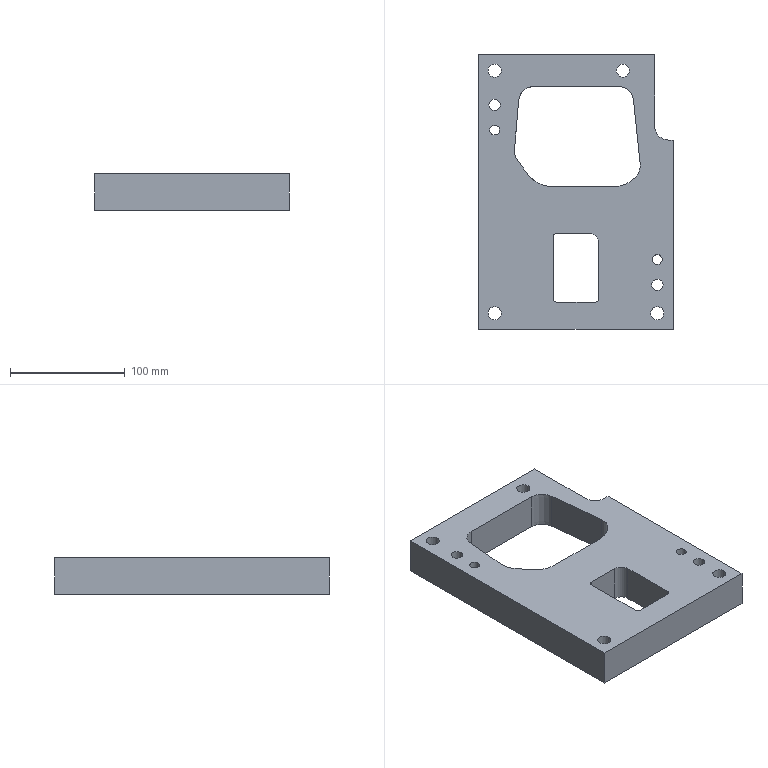Part | STEP file | lll_id3682_x_t | 1 solid | 45 faces | box 170 x 240 x 32 mm | volume 880662 mm3 | plane 22 | cylinder 19 | other 4 | commonest cylinder face diameters 11.509 x4 18.008 x4 6 x3 8.506 x2 10 x2 16 x1
STEP:
#1=CARTESIAN_POINT('',(3672.243,-109.5,60.5));
#2=VERTEX_POINT('',#1);
#3=CARTESIAN_POINT('',(3668.,-109.5,60.5));
#4=VERTEX_POINT('',#3);
#5=CARTESIAN_POINT('',(3587.243,-109.5,60.5));
#6=DIRECTION('',(-1.,0.,0.));
#7=VECTOR('',#6,1.);
#8=LINE('',#5,#7);
#9=EDGE_CURVE('',#2,#4,#8,.T.);
#10=ORIENTED_EDGE('',*,*,#9,.F.);
#11=CARTESIAN_POINT('',(3672.243,-274.803,60.5));
#12=VERTEX_POINT('',#11);
#13=CARTESIAN_POINT('',(3672.243,-156.803,60.5));
#14=DIRECTION('',(0.,-1.,0.));
#15=VECTOR('',#14,1.);
#16=LINE('',#13,#15);
#17=EDGE_CURVE('',#2,#12,#16,.T.);
#18=ORIENTED_EDGE('',*,*,#17,.T.);
#19=CARTESIAN_POINT('',(3502.243,-274.803,60.5));
#20=VERTEX_POINT('',#19);
#21=CARTESIAN_POINT('',(3587.243,-274.803,60.5));
#22=DIRECTION('',(-1.,0.,0.));
#23=VECTOR('',#22,1.);
#24=LINE('',#21,#23);
#25=EDGE_CURVE('',#12,#20,#24,.T.);
#26=ORIENTED_EDGE('',*,*,#25,.T.);
#27=CARTESIAN_POINT('',(3502.243,-34.803,60.5));
#28=VERTEX_POINT('',#27);
#29=CARTESIAN_POINT('',(3502.243,-156.803,60.5));
#30=DIRECTION('',(0.,1.,0.));
#31=VECTOR('',#30,1.);
#32=LINE('',#29,#31);
#33=EDGE_CURVE('',#20,#28,#32,.T.);
#34=ORIENTED_EDGE('',*,*,#33,.T.);
#35=CARTESIAN_POINT('',(3656.,-34.803,60.5));
#36=VERTEX_POINT('',#35);
#37=CARTESIAN_POINT('',(3587.243,-34.803,60.5));
#38=DIRECTION('',(1.,0.,0.));
#39=VECTOR('',#38,1.);
#40=LINE('',#37,#39);
#41=EDGE_CURVE('',#28,#36,#40,.T.);
#42=ORIENTED_EDGE('',*,*,#41,.T.);
#43=CARTESIAN_POINT('',(3656.,-97.5,60.5));
#44=VERTEX_POINT('',#43);
#45=CARTESIAN_POINT('',(3656.,-156.803,60.5));
#46=DIRECTION('',(0.,1.,0.));
#47=VECTOR('',#46,1.);
#48=LINE('',#45,#47);
#49=EDGE_CURVE('',#44,#36,#48,.T.);
#50=ORIENTED_EDGE('',*,*,#49,.F.);
#51=CARTESIAN_POINT('',(3668.,-97.5,60.5));
#52=DIRECTION('',(0.,0.,1.));
#53=DIRECTION('',(-1.,0.,0.));
#54=AXIS2_PLACEMENT_3D('',#51,#52,#53);
#55=CIRCLE('',#54,12.);
#56=EDGE_CURVE('',#44,#4,#55,.T.);
#57=ORIENTED_EDGE('',*,*,#56,.T.);
#58=EDGE_LOOP('',(#10,#18,#26,#34,#42,#50,#57));
#59=FACE_BOUND('',#58,.T.);
#60=CARTESIAN_POINT('',(3511.99,-100.803,60.5));
#61=VERTEX_POINT('',#60);
#62=CARTESIAN_POINT('',(3516.243,-100.803,60.5));
#63=DIRECTION('',(0.,0.,-1.));
#64=DIRECTION('',(-1.,0.,0.));
#65=AXIS2_PLACEMENT_3D('',#62,#63,#64);
#66=CIRCLE('',#65,4.253);
#67=EDGE_CURVE('',#61,#61,#66,.T.);
#68=ORIENTED_EDGE('',*,*,#67,.F.);
#69=EDGE_LOOP('',(#68));
#70=FACE_BOUND('',#69,.T.);
#71=CARTESIAN_POINT('',(3521.244,-78.803,60.5));
#72=VERTEX_POINT('',#71);
#73=CARTESIAN_POINT('',(3516.243,-78.803,60.5));
#74=DIRECTION('',(0.,0.,1.));
#75=DIRECTION('',(1.,0.,0.));
#76=AXIS2_PLACEMENT_3D('',#73,#74,#75);
#77=CIRCLE('',#76,5.);
#78=EDGE_CURVE('',#72,#72,#77,.T.);
#79=ORIENTED_EDGE('',*,*,#78,.T.);
#80=EDGE_LOOP('',(#79));
#81=FACE_BOUND('',#80,.T.);
#82=CARTESIAN_POINT('',(3663.244,-235.803,60.5));
#83=VERTEX_POINT('',#82);
#84=CARTESIAN_POINT('',(3658.243,-235.803,60.5));
#85=DIRECTION('',(0.,0.,1.));
#86=DIRECTION('',(1.,0.,0.));
#87=AXIS2_PLACEMENT_3D('',#84,#85,#86);
#88=CIRCLE('',#87,5.);
#89=EDGE_CURVE('',#83,#83,#88,.T.);
#90=ORIENTED_EDGE('',*,*,#89,.T.);
#91=EDGE_LOOP('',(#90));
#92=FACE_BOUND('',#91,.T.);
#93=CARTESIAN_POINT('',(3507.239,-260.803,60.5));
#94=VERTEX_POINT('',#93);
#95=CARTESIAN_POINT('',(3516.243,-260.803,60.5));
#96=DIRECTION('',(0.,0.,-1.));
#97=DIRECTION('',(-1.,0.,0.));
#98=AXIS2_PLACEMENT_3D('',#95,#96,#97);
#99=CIRCLE('',#98,9.004);
#100=EDGE_CURVE('',#94,#94,#99,.T.);
#101=ORIENTED_EDGE('',*,*,#100,.F.);
#102=EDGE_LOOP('',(#101));
#103=FACE_BOUND('',#102,.T.);
#104=CARTESIAN_POINT('',(3649.239,-260.803,60.5));
#105=VERTEX_POINT('',#104);
#106=CARTESIAN_POINT('',(3658.243,-260.803,60.5));
#107=DIRECTION('',(0.,0.,-1.));
#108=DIRECTION('',(-1.,0.,0.));
#109=AXIS2_PLACEMENT_3D('',#106,#107,#108);
#110=CIRCLE('',#109,9.004);
#111=EDGE_CURVE('',#105,#105,#110,.T.);
#112=ORIENTED_EDGE('',*,*,#111,.F.);
#113=EDGE_LOOP('',(#112));
#114=FACE_BOUND('',#113,.T.);
#115=CARTESIAN_POINT('',(3507.239,-48.803,60.5));
#116=VERTEX_POINT('',#115);
#117=CARTESIAN_POINT('',(3516.243,-48.803,60.5));
#118=DIRECTION('',(0.,0.,-1.));
#119=DIRECTION('',(-1.,0.,0.));
#120=AXIS2_PLACEMENT_3D('',#117,#118,#119);
#121=CIRCLE('',#120,9.004);
#122=EDGE_CURVE('',#116,#116,#121,.T.);
#123=ORIENTED_EDGE('',*,*,#122,.F.);
#124=EDGE_LOOP('',(#123));
#125=FACE_BOUND('',#124,.T.);
#126=CARTESIAN_POINT('',(3619.239,-48.803,60.5));
#127=VERTEX_POINT('',#126);
#128=CARTESIAN_POINT('',(3628.243,-48.803,60.5));
#129=DIRECTION('',(0.,0.,-1.));
#130=DIRECTION('',(-1.,0.,0.));
#131=AXIS2_PLACEMENT_3D('',#128,#129,#130);
#132=CIRCLE('',#131,9.004);
#133=EDGE_CURVE('',#127,#127,#132,.T.);
#134=ORIENTED_EDGE('',*,*,#133,.F.);
#135=EDGE_LOOP('',(#134));
#136=FACE_BOUND('',#135,.T.);
#137=CARTESIAN_POINT('',(3653.99,-213.803,60.5));
#138=VERTEX_POINT('',#137);
#139=CARTESIAN_POINT('',(3658.243,-213.803,60.5));
#140=DIRECTION('',(0.,0.,-1.));
#141=DIRECTION('',(-1.,0.,0.));
#142=AXIS2_PLACEMENT_3D('',#139,#140,#141);
#143=CIRCLE('',#142,4.253);
#144=EDGE_CURVE('',#138,#138,#143,.T.);
#145=ORIENTED_EDGE('',*,*,#144,.F.);
#146=EDGE_LOOP('',(#145));
#147=FACE_BOUND('',#146,.T.);
#148=CARTESIAN_POINT('',(3607.234,-198.95,60.5));
#149=VERTEX_POINT('',#148);
#150=CARTESIAN_POINT('',(3607.234,-247.95,60.5));
#151=VERTEX_POINT('',#150);
#152=CARTESIAN_POINT('',(3607.234,-199.225,60.5));
#153=DIRECTION('',(0.,-1.,0.));
#154=VECTOR('',#153,1.);
#155=LINE('',#152,#154);
#156=EDGE_CURVE('',#149,#151,#155,.T.);
#157=ORIENTED_EDGE('',*,*,#156,.F.);
#158=CARTESIAN_POINT('',(3599.234,-190.95,60.5));
#159=VERTEX_POINT('',#158);
#160=CARTESIAN_POINT('',(3599.234,-198.95,60.5));
#161=DIRECTION('',(0.,0.,1.));
#162=DIRECTION('',(-1.,0.,0.));
#163=AXIS2_PLACEMENT_3D('',#160,#161,#162);
#164=CIRCLE('',#163,8.);
#165=EDGE_CURVE('',#149,#159,#164,.T.);
#166=ORIENTED_EDGE('',*,*,#165,.T.);
#167=CARTESIAN_POINT('',(3570.234,-190.95,60.5));
#168=VERTEX_POINT('',#167);
#169=CARTESIAN_POINT('',(3587.234,-190.95,60.5));
#170=DIRECTION('',(1.,0.,0.));
#171=VECTOR('',#170,1.);
#172=LINE('',#169,#171);
#173=EDGE_CURVE('',#168,#159,#172,.T.);
#174=ORIENTED_EDGE('',*,*,#173,.F.);
#175=CARTESIAN_POINT('',(3567.234,-193.95,60.5));
#176=VERTEX_POINT('',#175);
#177=CARTESIAN_POINT('',(3570.234,-193.95,60.5));
#178=DIRECTION('',(0.,0.,1.));
#179=DIRECTION('',(-1.,0.,0.));
#180=AXIS2_PLACEMENT_3D('',#177,#178,#179);
#181=CIRCLE('',#180,3.);
#182=EDGE_CURVE('',#168,#176,#181,.T.);
#183=ORIENTED_EDGE('',*,*,#182,.T.);
#184=CARTESIAN_POINT('',(3567.234,-247.95,60.5));
#185=VERTEX_POINT('',#184);
#186=CARTESIAN_POINT('',(3567.234,-199.225,60.5));
#187=DIRECTION('',(0.,1.,0.));
#188=VECTOR('',#187,1.);
#189=LINE('',#186,#188);
#190=EDGE_CURVE('',#185,#176,#189,.T.);
#191=ORIENTED_EDGE('',*,*,#190,.F.);
#192=CARTESIAN_POINT('',(3570.234,-250.95,60.5));
#193=VERTEX_POINT('',#192);
#194=CARTESIAN_POINT('',(3570.234,-247.95,60.5));
#195=DIRECTION('',(0.,0.,1.));
#196=DIRECTION('',(-1.,0.,0.));
#197=AXIS2_PLACEMENT_3D('',#194,#195,#196);
#198=CIRCLE('',#197,3.);
#199=EDGE_CURVE('',#185,#193,#198,.T.);
#200=ORIENTED_EDGE('',*,*,#199,.T.);
#201=CARTESIAN_POINT('',(3604.234,-250.95,60.5));
#202=VERTEX_POINT('',#201);
#203=CARTESIAN_POINT('',(3587.234,-250.95,60.5));
#204=DIRECTION('',(-1.,0.,0.));
#205=VECTOR('',#204,1.);
#206=LINE('',#203,#205);
#207=EDGE_CURVE('',#202,#193,#206,.T.);
#208=ORIENTED_EDGE('',*,*,#207,.F.);
#209=CARTESIAN_POINT('',(3604.234,-247.95,60.5));
#210=DIRECTION('',(0.,0.,1.));
#211=DIRECTION('',(-1.,0.,0.));
#212=AXIS2_PLACEMENT_3D('',#209,#210,#211);
#213=CIRCLE('',#212,3.);
#214=EDGE_CURVE('',#202,#151,#213,.T.);
#215=ORIENTED_EDGE('',*,*,#214,.T.);
#216=EDGE_LOOP('',(#157,#166,#174,#183,#191,#200,#208,#215));
#217=FACE_BOUND('',#216,.T.);
#218=CARTESIAN_POINT('',(3643.25,-130.089,60.5));
#219=VERTEX_POINT('',#218);
#220=CARTESIAN_POINT('',(3638.938,-142.263,60.5));
#221=VERTEX_POINT('',#220);
#222=CARTESIAN_POINT('',(3628.332,-131.657,60.5));
#223=DIRECTION('',(0.,0.,-1.));
#224=DIRECTION('',(-1.,0.,0.));
#225=AXIS2_PLACEMENT_3D('',#222,#223,#224);
#226=CIRCLE('',#225,15.);
#227=EDGE_CURVE('',#219,#221,#226,.T.);
#228=ORIENTED_EDGE('',*,*,#227,.F.);
#229=CARTESIAN_POINT('',(3637.367,-74.119,60.5));
#230=VERTEX_POINT('',#229);
#231=CARTESIAN_POINT('',(3645.415,-150.689,60.5));
#232=DIRECTION('',(0.1045,-0.9945,0.));
#233=VECTOR('',#232,1.);
#234=LINE('',#231,#233);
#235=EDGE_CURVE('',#230,#219,#234,.T.);
#236=ORIENTED_EDGE('',*,*,#235,.F.);
#237=CARTESIAN_POINT('',(3624.637,-62.657,60.5));
#238=VERTEX_POINT('',#237);
#239=CARTESIAN_POINT('',(3624.637,-62.657,60.5));
#240=CARTESIAN_POINT('',(3627.791,-62.657,60.5));
#241=CARTESIAN_POINT('',(3630.87,-63.847,60.5));
#242=CARTESIAN_POINT('',(3635.525,-68.034,60.5));
#243=CARTESIAN_POINT('',(3637.037,-70.978,60.5));
#244=CARTESIAN_POINT('',(3637.367,-74.119,60.5));
#245=B_SPLINE_CURVE_WITH_KNOTS('',3,(#239,#240,#241,#242,#243,#244),.UNSPECIFIED.,.F.,.F.,(4,2,4),(0.,0.5,1.),.UNSPECIFIED.);
#246=EDGE_CURVE('',#238,#230,#245,.T.);
#247=ORIENTED_EDGE('',*,*,#246,.F.);
#248=CARTESIAN_POINT('',(3550.037,-62.657,60.5));
#249=VERTEX_POINT('',#248);
#250=CARTESIAN_POINT('',(3587.243,-62.657,60.5));
#251=DIRECTION('',(1.,0.,0.));
#252=VECTOR('',#251,1.);
#253=LINE('',#250,#252);
#254=EDGE_CURVE('',#249,#238,#253,.T.);
#255=ORIENTED_EDGE('',*,*,#254,.F.);
#256=CARTESIAN_POINT('',(3537.286,-74.341,60.5));
#257=VERTEX_POINT('',#256);
#258=CARTESIAN_POINT('',(3537.286,-74.341,60.5));
#259=CARTESIAN_POINT('',(3537.564,-71.162,60.5));
#260=CARTESIAN_POINT('',(3539.052,-68.163,60.5));
#261=CARTESIAN_POINT('',(3543.717,-63.885,60.5));
#262=CARTESIAN_POINT('',(3546.842,-62.657,60.5));
#263=CARTESIAN_POINT('',(3550.037,-62.657,60.5));
#264=B_SPLINE_CURVE_WITH_KNOTS('',3,(#258,#259,#260,#261,#262,#263),.UNSPECIFIED.,.F.,.F.,(4,2,4),(0.,0.5,1.),.UNSPECIFIED.);
#265=EDGE_CURVE('',#257,#249,#264,.T.);
#266=ORIENTED_EDGE('',*,*,#265,.F.);
#267=CARTESIAN_POINT('',(3533.523,-117.349,60.5));
#268=VERTEX_POINT('',#267);
#269=CARTESIAN_POINT('',(3530.506,-151.839,60.5));
#270=DIRECTION('',(0.08716,0.9962,0.));
#271=VECTOR('',#270,1.);
#272=LINE('',#269,#271);
#273=EDGE_CURVE('',#268,#257,#272,.T.);
#274=ORIENTED_EDGE('',*,*,#273,.F.);
#275=CARTESIAN_POINT('',(3536.486,-127.684,60.5));
#276=VERTEX_POINT('',#275);
#277=CARTESIAN_POINT('',(3536.486,-127.684,60.5));
#278=CARTESIAN_POINT('',(3534.267,-124.738,60.5));
#279=CARTESIAN_POINT('',(3533.202,-121.023,60.5));
#280=CARTESIAN_POINT('',(3533.523,-117.349,60.5));
#281=B_SPLINE_CURVE_WITH_KNOTS('',3,(#277,#278,#279,#280),.UNSPECIFIED.,.F.,.F.,(4,4),(0.,1.),.UNSPECIFIED.);
#282=EDGE_CURVE('',#276,#268,#281,.T.);
#283=ORIENTED_EDGE('',*,*,#282,.F.);
#284=CARTESIAN_POINT('',(3545.814,-140.062,60.5));
#285=VERTEX_POINT('',#284);
#286=CARTESIAN_POINT('',(3568.865,-170.652,60.5));
#287=DIRECTION('',(-0.6018,0.7986,0.));
#288=VECTOR('',#287,1.);
#289=LINE('',#286,#288);
#290=EDGE_CURVE('',#285,#276,#289,.T.);
#291=ORIENTED_EDGE('',*,*,#290,.F.);
#292=CARTESIAN_POINT('',(3565.78,-150.017,60.5));
#293=VERTEX_POINT('',#292);
#294=CARTESIAN_POINT('',(3565.78,-150.017,60.5));
#295=CARTESIAN_POINT('',(3561.891,-150.017,60.5));
#296=CARTESIAN_POINT('',(3558.048,-149.099,60.5));
#297=CARTESIAN_POINT('',(3552.892,-146.525,60.5));
#298=CARTESIAN_POINT('',(3551.245,-145.458,60.5));
#299=CARTESIAN_POINT('',(3548.301,-143.006,60.5));
#300=CARTESIAN_POINT('',(3546.983,-141.614,60.5));
#301=CARTESIAN_POINT('',(3545.814,-140.062,60.5));
#302=B_SPLINE_CURVE_WITH_KNOTS('',3,(#294,#295,#296,#297,#298,#299,#300,#301),.UNSPECIFIED.,.F.,.F.,(4,2,2,4),(0.,0.5,0.75,1.),.UNSPECIFIED.);
#303=EDGE_CURVE('',#293,#285,#302,.T.);
#304=ORIENTED_EDGE('',*,*,#303,.F.);
#305=CARTESIAN_POINT('',(3620.83,-150.017,60.5));
#306=VERTEX_POINT('',#305);
#307=CARTESIAN_POINT('',(3587.243,-150.017,60.5));
#308=DIRECTION('',(-1.,0.,0.));
#309=VECTOR('',#308,1.);
#310=LINE('',#307,#309);
#311=EDGE_CURVE('',#306,#293,#310,.T.);
#312=ORIENTED_EDGE('',*,*,#311,.F.);
#313=CARTESIAN_POINT('',(3638.507,-142.694,60.5));
#314=VERTEX_POINT('',#313);
#315=CARTESIAN_POINT('',(3620.83,-125.017,60.5));
#316=DIRECTION('',(0.,0.,-1.));
#317=DIRECTION('',(-1.,0.,0.));
#318=AXIS2_PLACEMENT_3D('',#315,#316,#317);
#319=CIRCLE('',#318,25.);
#320=EDGE_CURVE('',#314,#306,#319,.T.);
#321=ORIENTED_EDGE('',*,*,#320,.F.);
#322=CARTESIAN_POINT('',(3605.821,-175.381,60.5));
#323=DIRECTION('',(0.7071,0.7071,0.));
#324=VECTOR('',#323,1.);
#325=LINE('',#322,#324);
#326=EDGE_CURVE('',#314,#221,#325,.T.);
#327=ORIENTED_EDGE('',*,*,#326,.T.);
#328=EDGE_LOOP('',(#228,#236,#247,#255,#266,#274,#283,#291,#304,#312,#321,#327));
#329=FACE_BOUND('',#328,.T.);
#330=CARTESIAN_POINT('',(3587.243,-156.803,60.5));
#331=DIRECTION('',(0.,0.,-1.));
#332=DIRECTION('',(1.,0.,0.));
#333=AXIS2_PLACEMENT_3D('',#330,#331,#332);
#334=PLANE('',#333);
#335=ADVANCED_FACE('',(#59,#70,#81,#92,#103,#114,#125,#136,#147,#217,#329),#334,.T.);
#336=CARTESIAN_POINT('',(3656.,-34.803,92.5));
#337=VERTEX_POINT('',#336);
#338=CARTESIAN_POINT('',(3656.,-97.5,92.5));
#339=VERTEX_POINT('',#338);
#340=CARTESIAN_POINT('',(3656.,-156.803,92.5));
#341=DIRECTION('',(0.,-1.,0.));
#342=VECTOR('',#341,1.);
#343=LINE('',#340,#342);
#344=EDGE_CURVE('',#337,#339,#343,.T.);
#345=ORIENTED_EDGE('',*,*,#344,.F.);
#346=CARTESIAN_POINT('',(3502.243,-34.803,92.5));
#347=VERTEX_POINT('',#346);
#348=CARTESIAN_POINT('',(3587.243,-34.803,92.5));
#349=DIRECTION('',(-1.,0.,0.));
#350=VECTOR('',#349,1.);
#351=LINE('',#348,#350);
#352=EDGE_CURVE('',#337,#347,#351,.T.);
#353=ORIENTED_EDGE('',*,*,#352,.T.);
#354=CARTESIAN_POINT('',(3502.243,-274.803,92.5));
#355=VERTEX_POINT('',#354);
#356=CARTESIAN_POINT('',(3502.243,-156.803,92.5));
#357=DIRECTION('',(0.,-1.,0.));
#358=VECTOR('',#357,1.);
#359=LINE('',#356,#358);
#360=EDGE_CURVE('',#347,#355,#359,.T.);
#361=ORIENTED_EDGE('',*,*,#360,.T.);
#362=CARTESIAN_POINT('',(3672.243,-274.803,92.5));
#363=VERTEX_POINT('',#362);
#364=CARTESIAN_POINT('',(3587.243,-274.803,92.5));
#365=DIRECTION('',(1.,0.,0.));
#366=VECTOR('',#365,1.);
#367=LINE('',#364,#366);
#368=EDGE_CURVE('',#355,#363,#367,.T.);
#369=ORIENTED_EDGE('',*,*,#368,.T.);
#370=CARTESIAN_POINT('',(3672.243,-109.5,92.5));
#371=VERTEX_POINT('',#370);
#372=CARTESIAN_POINT('',(3672.243,-156.803,92.5));
#373=DIRECTION('',(0.,1.,0.));
#374=VECTOR('',#373,1.);
#375=LINE('',#372,#374);
#376=EDGE_CURVE('',#363,#371,#375,.T.);
#377=ORIENTED_EDGE('',*,*,#376,.T.);
#378=CARTESIAN_POINT('',(3668.,-109.5,92.5));
#379=VERTEX_POINT('',#378);
#380=CARTESIAN_POINT('',(3587.243,-109.5,92.5));
#381=DIRECTION('',(1.,0.,0.));
#382=VECTOR('',#381,1.);
#383=LINE('',#380,#382);
#384=EDGE_CURVE('',#379,#371,#383,.T.);
#385=ORIENTED_EDGE('',*,*,#384,.F.);
#386=CARTESIAN_POINT('',(3668.,-97.5,92.5));
#387=DIRECTION('',(0.,0.,-1.));
#388=DIRECTION('',(1.,0.,0.));
#389=AXIS2_PLACEMENT_3D('',#386,#387,#388);
#390=CIRCLE('',#389,12.);
#391=EDGE_CURVE('',#379,#339,#390,.T.);
#392=ORIENTED_EDGE('',*,*,#391,.T.);
#393=EDGE_LOOP('',(#345,#353,#361,#369,#377,#385,#392));
#394=FACE_BOUND('',#393,.T.);
#395=CARTESIAN_POINT('',(3653.99,-213.803,92.5));
#396=VERTEX_POINT('',#395);
#397=CARTESIAN_POINT('',(3658.243,-213.803,92.5));
#398=DIRECTION('',(0.,0.,-1.));
#399=DIRECTION('',(-1.,0.,0.));
#400=AXIS2_PLACEMENT_3D('',#397,#398,#399);
#401=CIRCLE('',#400,4.253);
#402=EDGE_CURVE('',#396,#396,#401,.T.);
#403=ORIENTED_EDGE('',*,*,#402,.T.);
#404=EDGE_LOOP('',(#403));
#405=FACE_BOUND('',#404,.T.);
#406=CARTESIAN_POINT('',(3511.99,-100.803,92.5));
#407=VERTEX_POINT('',#406);
#408=CARTESIAN_POINT('',(3516.243,-100.803,92.5));
#409=DIRECTION('',(0.,0.,-1.));
#410=DIRECTION('',(-1.,0.,0.));
#411=AXIS2_PLACEMENT_3D('',#408,#409,#410);
#412=CIRCLE('',#411,4.253);
#413=EDGE_CURVE('',#407,#407,#412,.T.);
#414=ORIENTED_EDGE('',*,*,#413,.T.);
#415=EDGE_LOOP('',(#414));
#416=FACE_BOUND('',#415,.T.);
#417=CARTESIAN_POINT('',(3511.243,-78.803,92.5));
#418=VERTEX_POINT('',#417);
#419=CARTESIAN_POINT('',(3516.243,-78.803,92.5));
#420=DIRECTION('',(0.,0.,-1.));
#421=DIRECTION('',(-1.,0.,0.));
#422=AXIS2_PLACEMENT_3D('',#419,#420,#421);
#423=CIRCLE('',#422,5.);
#424=EDGE_CURVE('',#418,#418,#423,.T.);
#425=ORIENTED_EDGE('',*,*,#424,.T.);
#426=EDGE_LOOP('',(#425));
#427=FACE_BOUND('',#426,.T.);
#428=CARTESIAN_POINT('',(3653.243,-235.803,92.5));
#429=VERTEX_POINT('',#428);
#430=CARTESIAN_POINT('',(3658.243,-235.803,92.5));
#431=DIRECTION('',(0.,0.,-1.));
#432=DIRECTION('',(-1.,0.,0.));
#433=AXIS2_PLACEMENT_3D('',#430,#431,#432);
#434=CIRCLE('',#433,5.);
#435=EDGE_CURVE('',#429,#429,#434,.T.);
#436=ORIENTED_EDGE('',*,*,#435,.T.);
#437=EDGE_LOOP('',(#436));
#438=FACE_BOUND('',#437,.T.);
#439=CARTESIAN_POINT('',(3622.489,-48.803,92.5));
#440=VERTEX_POINT('',#439);
#441=CARTESIAN_POINT('',(3628.243,-48.803,92.5));
#442=DIRECTION('',(0.,0.,-1.));
#443=DIRECTION('',(-1.,0.,0.));
#444=AXIS2_PLACEMENT_3D('',#441,#442,#443);
#445=CIRCLE('',#444,5.755);
#446=EDGE_CURVE('',#440,#440,#445,.T.);
#447=ORIENTED_EDGE('',*,*,#446,.T.);
#448=EDGE_LOOP('',(#447));
#449=FACE_BOUND('',#448,.T.);
#450=CARTESIAN_POINT('',(3510.489,-260.803,92.5));
#451=VERTEX_POINT('',#450);
#452=CARTESIAN_POINT('',(3516.243,-260.803,92.5));
#453=DIRECTION('',(0.,0.,-1.));
#454=DIRECTION('',(-1.,0.,0.));
#455=AXIS2_PLACEMENT_3D('',#452,#453,#454);
#456=CIRCLE('',#455,5.755);
#457=EDGE_CURVE('',#451,#451,#456,.T.);
#458=ORIENTED_EDGE('',*,*,#457,.T.);
#459=EDGE_LOOP('',(#458));
#460=FACE_BOUND('',#459,.T.);
#461=CARTESIAN_POINT('',(3510.489,-48.803,92.5));
#462=VERTEX_POINT('',#461);
#463=CARTESIAN_POINT('',(3516.243,-48.803,92.5));
#464=DIRECTION('',(0.,0.,-1.));
#465=DIRECTION('',(-1.,0.,0.));
#466=AXIS2_PLACEMENT_3D('',#463,#464,#465);
#467=CIRCLE('',#466,5.755);
#468=EDGE_CURVE('',#462,#462,#467,.T.);
#469=ORIENTED_EDGE('',*,*,#468,.T.);
#470=EDGE_LOOP('',(#469));
#471=FACE_BOUND('',#470,.T.);
#472=CARTESIAN_POINT('',(3652.489,-260.803,92.5));
#473=VERTEX_POINT('',#472);
#474=CARTESIAN_POINT('',(3658.243,-260.803,92.5));
#475=DIRECTION('',(0.,0.,-1.));
#476=DIRECTION('',(-1.,0.,0.));
#477=AXIS2_PLACEMENT_3D('',#474,#475,#476);
#478=CIRCLE('',#477,5.755);
#479=EDGE_CURVE('',#473,#473,#478,.T.);
#480=ORIENTED_EDGE('',*,*,#479,.T.);
#481=EDGE_LOOP('',(#480));
#482=FACE_BOUND('',#481,.T.);
#483=CARTESIAN_POINT('',(3599.234,-190.95,92.5));
#484=VERTEX_POINT('',#483);
#485=CARTESIAN_POINT('',(3570.234,-190.95,92.5));
#486=VERTEX_POINT('',#485);
#487=CARTESIAN_POINT('',(3587.234,-190.95,92.5));
#488=DIRECTION('',(-1.,0.,0.));
#489=VECTOR('',#488,1.);
#490=LINE('',#487,#489);
#491=EDGE_CURVE('',#484,#486,#490,.T.);
#492=ORIENTED_EDGE('',*,*,#491,.F.);
#493=CARTESIAN_POINT('',(3607.234,-198.95,92.5));
#494=VERTEX_POINT('',#493);
#495=CARTESIAN_POINT('',(3599.234,-198.95,92.5));
#496=DIRECTION('',(0.,0.,-1.));
#497=DIRECTION('',(1.,0.,0.));
#498=AXIS2_PLACEMENT_3D('',#495,#496,#497);
#499=CIRCLE('',#498,8.);
#500=EDGE_CURVE('',#484,#494,#499,.T.);
#501=ORIENTED_EDGE('',*,*,#500,.T.);
#502=CARTESIAN_POINT('',(3607.234,-247.95,92.5));
#503=VERTEX_POINT('',#502);
#504=CARTESIAN_POINT('',(3607.234,-199.225,92.5));
#505=DIRECTION('',(0.,1.,0.));
#506=VECTOR('',#505,1.);
#507=LINE('',#504,#506);
#508=EDGE_CURVE('',#503,#494,#507,.T.);
#509=ORIENTED_EDGE('',*,*,#508,.F.);
#510=CARTESIAN_POINT('',(3604.234,-250.95,92.5));
#511=VERTEX_POINT('',#510);
#512=CARTESIAN_POINT('',(3604.234,-247.95,92.5));
#513=DIRECTION('',(0.,0.,-1.));
#514=DIRECTION('',(1.,0.,0.));
#515=AXIS2_PLACEMENT_3D('',#512,#513,#514);
#516=CIRCLE('',#515,3.);
#517=EDGE_CURVE('',#503,#511,#516,.T.);
#518=ORIENTED_EDGE('',*,*,#517,.T.);
#519=CARTESIAN_POINT('',(3570.234,-250.95,92.5));
#520=VERTEX_POINT('',#519);
#521=CARTESIAN_POINT('',(3587.234,-250.95,92.5));
#522=DIRECTION('',(1.,0.,0.));
#523=VECTOR('',#522,1.);
#524=LINE('',#521,#523);
#525=EDGE_CURVE('',#520,#511,#524,.T.);
#526=ORIENTED_EDGE('',*,*,#525,.F.);
#527=CARTESIAN_POINT('',(3567.234,-247.95,92.5));
#528=VERTEX_POINT('',#527);
#529=CARTESIAN_POINT('',(3570.234,-247.95,92.5));
#530=DIRECTION('',(0.,0.,-1.));
#531=DIRECTION('',(1.,0.,0.));
#532=AXIS2_PLACEMENT_3D('',#529,#530,#531);
#533=CIRCLE('',#532,3.);
#534=EDGE_CURVE('',#520,#528,#533,.T.);
#535=ORIENTED_EDGE('',*,*,#534,.T.);
#536=CARTESIAN_POINT('',(3567.234,-193.95,92.5));
#537=VERTEX_POINT('',#536);
#538=CARTESIAN_POINT('',(3567.234,-199.225,92.5));
#539=DIRECTION('',(0.,-1.,0.));
#540=VECTOR('',#539,1.);
#541=LINE('',#538,#540);
#542=EDGE_CURVE('',#537,#528,#541,.T.);
#543=ORIENTED_EDGE('',*,*,#542,.F.);
#544=CARTESIAN_POINT('',(3570.234,-193.95,92.5));
#545=DIRECTION('',(0.,0.,-1.));
#546=DIRECTION('',(1.,0.,0.));
#547=AXIS2_PLACEMENT_3D('',#544,#545,#546);
#548=CIRCLE('',#547,3.);
#549=EDGE_CURVE('',#537,#486,#548,.T.);
#550=ORIENTED_EDGE('',*,*,#549,.T.);
#551=EDGE_LOOP('',(#492,#501,#509,#518,#526,#535,#543,#550));
#552=FACE_BOUND('',#551,.T.);
#553=CARTESIAN_POINT('',(3620.83,-150.017,92.5));
#554=VERTEX_POINT('',#553);
#555=CARTESIAN_POINT('',(3638.507,-142.694,92.5));
#556=VERTEX_POINT('',#555);
#557=CARTESIAN_POINT('',(3620.83,-125.017,92.5));
#558=DIRECTION('',(0.,0.,1.));
#559=DIRECTION('',(1.,0.,0.));
#560=AXIS2_PLACEMENT_3D('',#557,#558,#559);
#561=CIRCLE('',#560,25.);
#562=EDGE_CURVE('',#554,#556,#561,.T.);
#563=ORIENTED_EDGE('',*,*,#562,.F.);
#564=CARTESIAN_POINT('',(3565.78,-150.017,92.5));
#565=VERTEX_POINT('',#564);
#566=CARTESIAN_POINT('',(3587.243,-150.017,92.5));
#567=DIRECTION('',(1.,0.,0.));
#568=VECTOR('',#567,1.);
#569=LINE('',#566,#568);
#570=EDGE_CURVE('',#565,#554,#569,.T.);
#571=ORIENTED_EDGE('',*,*,#570,.F.);
#572=CARTESIAN_POINT('',(3545.814,-140.062,92.5));
#573=VERTEX_POINT('',#572);
#574=CARTESIAN_POINT('',(3545.814,-140.062,92.5));
#575=CARTESIAN_POINT('',(3548.154,-143.168,92.5));
#576=CARTESIAN_POINT('',(3551.2,-145.685,92.5));
#577=CARTESIAN_POINT('',(3556.359,-148.253,92.5));
#578=CARTESIAN_POINT('',(3558.202,-148.927,92.5));
#579=CARTESIAN_POINT('',(3561.932,-149.802,92.5));
#580=CARTESIAN_POINT('',(3563.837,-150.017,92.5));
#581=CARTESIAN_POINT('',(3565.78,-150.017,92.5));
#582=B_SPLINE_CURVE_WITH_KNOTS('',3,(#574,#575,#576,#577,#578,#579,#580,#581),.UNSPECIFIED.,.F.,.F.,(4,2,2,4),(0.,0.5,0.75,1.),.UNSPECIFIED.);
#583=EDGE_CURVE('',#573,#565,#582,.T.);
#584=ORIENTED_EDGE('',*,*,#583,.F.);
#585=CARTESIAN_POINT('',(3536.486,-127.684,92.5));
#586=VERTEX_POINT('',#585);
#587=CARTESIAN_POINT('',(3568.865,-170.652,92.5));
#588=DIRECTION('',(0.6018,-0.7986,0.));
#589=VECTOR('',#588,1.);
#590=LINE('',#587,#589);
#591=EDGE_CURVE('',#586,#573,#590,.T.);
#592=ORIENTED_EDGE('',*,*,#591,.F.);
#593=CARTESIAN_POINT('',(3533.523,-117.349,92.5));
#594=VERTEX_POINT('',#593);
#595=CARTESIAN_POINT('',(3533.523,-117.349,92.5));
#596=CARTESIAN_POINT('',(3533.202,-121.023,92.5));
#597=CARTESIAN_POINT('',(3534.267,-124.739,92.5));
#598=CARTESIAN_POINT('',(3536.486,-127.684,92.5));
#599=B_SPLINE_CURVE_WITH_KNOTS('',3,(#595,#596,#597,#598),.UNSPECIFIED.,.F.,.F.,(4,4),(0.,1.),.UNSPECIFIED.);
#600=EDGE_CURVE('',#594,#586,#599,.T.);
#601=ORIENTED_EDGE('',*,*,#600,.F.);
#602=CARTESIAN_POINT('',(3537.286,-74.341,92.5));
#603=VERTEX_POINT('',#602);
#604=CARTESIAN_POINT('',(3530.506,-151.839,92.5));
#605=DIRECTION('',(-0.08716,-0.9962,0.));
#606=VECTOR('',#605,1.);
#607=LINE('',#604,#606);
#608=EDGE_CURVE('',#603,#594,#607,.T.);
#609=ORIENTED_EDGE('',*,*,#608,.F.);
#610=CARTESIAN_POINT('',(3550.037,-62.657,92.5));
#611=VERTEX_POINT('',#610);
#612=CARTESIAN_POINT('',(3550.037,-62.657,92.5));
#613=CARTESIAN_POINT('',(3546.846,-62.657,92.5));
#614=CARTESIAN_POINT('',(3543.729,-63.878,92.5));
#615=CARTESIAN_POINT('',(3539.06,-68.152,92.5));
#616=CARTESIAN_POINT('',(3537.564,-71.158,92.5));
#617=CARTESIAN_POINT('',(3537.286,-74.341,92.5));
#618=B_SPLINE_CURVE_WITH_KNOTS('',3,(#612,#613,#614,#615,#616,#617),.UNSPECIFIED.,.F.,.F.,(4,2,4),(0.,0.5,1.),.UNSPECIFIED.);
#619=EDGE_CURVE('',#611,#603,#618,.T.);
#620=ORIENTED_EDGE('',*,*,#619,.F.);
#621=CARTESIAN_POINT('',(3624.637,-62.657,92.5));
#622=VERTEX_POINT('',#621);
#623=CARTESIAN_POINT('',(3587.243,-62.657,92.5));
#624=DIRECTION('',(-1.,0.,0.));
#625=VECTOR('',#624,1.);
#626=LINE('',#623,#625);
#627=EDGE_CURVE('',#622,#611,#626,.T.);
#628=ORIENTED_EDGE('',*,*,#627,.F.);
#629=CARTESIAN_POINT('',(3637.367,-74.119,92.5));
#630=VERTEX_POINT('',#629);
#631=CARTESIAN_POINT('',(3637.367,-74.119,92.5));
#632=CARTESIAN_POINT('',(3637.037,-70.982,92.5));
#633=CARTESIAN_POINT('',(3635.532,-68.044,92.5));
#634=CARTESIAN_POINT('',(3630.881,-63.852,92.5));
#635=CARTESIAN_POINT('',(3627.795,-62.657,92.5));
#636=CARTESIAN_POINT('',(3624.637,-62.657,92.5));
#637=B_SPLINE_CURVE_WITH_KNOTS('',3,(#631,#632,#633,#634,#635,#636),.UNSPECIFIED.,.F.,.F.,(4,2,4),(0.,0.5,1.),.UNSPECIFIED.);
#638=EDGE_CURVE('',#630,#622,#637,.T.);
#639=ORIENTED_EDGE('',*,*,#638,.F.);
#640=CARTESIAN_POINT('',(3643.25,-130.089,92.5));
#641=VERTEX_POINT('',#640);
#642=CARTESIAN_POINT('',(3645.415,-150.689,92.5));
#643=DIRECTION('',(-0.1045,0.9945,0.));
#644=VECTOR('',#643,1.);
#645=LINE('',#642,#644);
#646=EDGE_CURVE('',#641,#630,#645,.T.);
#647=ORIENTED_EDGE('',*,*,#646,.F.);
#648=CARTESIAN_POINT('',(3638.938,-142.263,92.5));
#649=VERTEX_POINT('',#648);
#650=CARTESIAN_POINT('',(3628.332,-131.657,92.5));
#651=DIRECTION('',(0.,0.,1.));
#652=DIRECTION('',(1.,0.,0.));
#653=AXIS2_PLACEMENT_3D('',#650,#651,#652);
#654=CIRCLE('',#653,15.);
#655=EDGE_CURVE('',#649,#641,#654,.T.);
#656=ORIENTED_EDGE('',*,*,#655,.F.);
#657=CARTESIAN_POINT('',(3802.568,21.366,92.5));
#658=DIRECTION('',(-0.7071,-0.7071,0.));
#659=VECTOR('',#658,1.);
#660=LINE('',#657,#659);
#661=EDGE_CURVE('',#649,#556,#660,.T.);
#662=ORIENTED_EDGE('',*,*,#661,.T.);
#663=EDGE_LOOP('',(#563,#571,#584,#592,#601,#609,#620,#628,#639,#647,#656,#662));
#664=FACE_BOUND('',#663,.T.);
#665=CARTESIAN_POINT('',(3587.243,-156.803,92.5));
#666=DIRECTION('',(0.,0.,1.));
#667=DIRECTION('',(-1.,0.,0.));
#668=AXIS2_PLACEMENT_3D('',#665,#666,#667);
#669=PLANE('',#668);
#670=ADVANCED_FACE('',(#394,#405,#416,#427,#438,#449,#460,#471,#482,#552,#664),#669,.T.);
#671=CARTESIAN_POINT('',(3672.243,-109.5,60.5));
#672=DIRECTION('',(0.,0.,1.));
#673=VECTOR('',#672,1.);
#674=LINE('',#671,#673);
#675=EDGE_CURVE('',#2,#371,#674,.T.);
#676=ORIENTED_EDGE('',*,*,#675,.T.);
#677=ORIENTED_EDGE('',*,*,#376,.F.);
#678=CARTESIAN_POINT('',(3672.243,-274.803,60.5));
#679=DIRECTION('',(0.,0.,1.));
#680=VECTOR('',#679,1.);
#681=LINE('',#678,#680);
#682=EDGE_CURVE('',#12,#363,#681,.T.);
#683=ORIENTED_EDGE('',*,*,#682,.F.);
#684=ORIENTED_EDGE('',*,*,#17,.F.);
#685=EDGE_LOOP('',(#676,#677,#683,#684));
#686=FACE_OUTER_BOUND('',#685,.T.);
#687=CARTESIAN_POINT('',(3672.243,-156.803,60.5));
#688=DIRECTION('',(1.,0.,0.));
#689=DIRECTION('',(0.,0.,1.));
#690=AXIS2_PLACEMENT_3D('',#687,#688,#689);
#691=PLANE('',#690);
#692=ADVANCED_FACE('',(#686),#691,.T.);
#693=CARTESIAN_POINT('',(3502.243,-274.803,60.5));
#694=DIRECTION('',(0.,0.,1.));
#695=VECTOR('',#694,1.);
#696=LINE('',#693,#695);
#697=EDGE_CURVE('',#20,#355,#696,.T.);
#698=ORIENTED_EDGE('',*,*,#697,.F.);
#699=ORIENTED_EDGE('',*,*,#25,.F.);
#700=ORIENTED_EDGE('',*,*,#682,.T.);
#701=ORIENTED_EDGE('',*,*,#368,.F.);
#702=EDGE_LOOP('',(#698,#699,#700,#701));
#703=FACE_OUTER_BOUND('',#702,.T.);
#704=CARTESIAN_POINT('',(3587.243,-274.803,60.5));
#705=DIRECTION('',(0.,-1.,0.));
#706=DIRECTION('',(0.,0.,-1.));
#707=AXIS2_PLACEMENT_3D('',#704,#705,#706);
#708=PLANE('',#707);
#709=ADVANCED_FACE('',(#703),#708,.T.);
#710=CARTESIAN_POINT('',(3656.,-34.803,60.5));
#711=DIRECTION('',(0.,0.,-1.));
#712=VECTOR('',#711,1.);
#713=LINE('',#710,#712);
#714=EDGE_CURVE('',#337,#36,#713,.T.);
#715=ORIENTED_EDGE('',*,*,#714,.T.);
#716=ORIENTED_EDGE('',*,*,#41,.F.);
#717=CARTESIAN_POINT('',(3502.243,-34.803,60.5));
#718=DIRECTION('',(0.,0.,1.));
#719=VECTOR('',#718,1.);
#720=LINE('',#717,#719);
#721=EDGE_CURVE('',#28,#347,#720,.T.);
#722=ORIENTED_EDGE('',*,*,#721,.T.);
#723=ORIENTED_EDGE('',*,*,#352,.F.);
#724=EDGE_LOOP('',(#715,#716,#722,#723));
#725=FACE_OUTER_BOUND('',#724,.T.);
#726=CARTESIAN_POINT('',(3587.243,-34.803,60.5));
#727=DIRECTION('',(0.,1.,0.));
#728=DIRECTION('',(0.,0.,1.));
#729=AXIS2_PLACEMENT_3D('',#726,#727,#728);
#730=PLANE('',#729);
#731=ADVANCED_FACE('',(#725),#730,.T.);
#732=ORIENTED_EDGE('',*,*,#33,.F.);
#733=ORIENTED_EDGE('',*,*,#697,.T.);
#734=ORIENTED_EDGE('',*,*,#360,.F.);
#735=ORIENTED_EDGE('',*,*,#721,.F.);
#736=EDGE_LOOP('',(#732,#733,#734,#735));
#737=FACE_OUTER_BOUND('',#736,.T.);
#738=CARTESIAN_POINT('',(3502.243,-156.803,60.5));
#739=DIRECTION('',(-1.,0.,0.));
#740=DIRECTION('',(0.,0.,-1.));
#741=AXIS2_PLACEMENT_3D('',#738,#739,#740);
#742=PLANE('',#741);
#743=ADVANCED_FACE('',(#737),#742,.T.);
#744=ORIENTED_EDGE('',*,*,#479,.F.);
#745=EDGE_LOOP('',(#744));
#746=FACE_BOUND('',#745,.T.);
#747=CARTESIAN_POINT('',(3652.489,-260.803,73.5));
#748=VERTEX_POINT('',#747);
#749=CARTESIAN_POINT('',(3658.243,-260.803,73.5));
#750=DIRECTION('',(0.,0.,-1.));
#751=DIRECTION('',(-1.,0.,0.));
#752=AXIS2_PLACEMENT_3D('',#749,#750,#751);
#753=CIRCLE('',#752,5.755);
#754=EDGE_CURVE('',#748,#748,#753,.T.);
#755=ORIENTED_EDGE('',*,*,#754,.T.);
#756=EDGE_LOOP('',(#755));
#757=FACE_BOUND('',#756,.T.);
#758=CARTESIAN_POINT('',(3658.243,-260.803,57.5));
#759=DIRECTION('',(0.,0.,1.));
#760=DIRECTION('',(-1.,0.,0.));
#761=AXIS2_PLACEMENT_3D('',#758,#759,#760);
#762=CYLINDRICAL_SURFACE('',#761,5.755);
#763=ADVANCED_FACE('',(#746,#757),#762,.F.);
#764=ORIENTED_EDGE('',*,*,#754,.F.);
#765=EDGE_LOOP('',(#764));
#766=FACE_BOUND('',#765,.T.);
#767=CARTESIAN_POINT('',(3649.239,-260.803,73.5));
#768=VERTEX_POINT('',#767);
#769=CARTESIAN_POINT('',(3658.243,-260.803,73.5));
#770=DIRECTION('',(0.,0.,-1.));
#771=DIRECTION('',(-1.,0.,0.));
#772=AXIS2_PLACEMENT_3D('',#769,#770,#771);
#773=CIRCLE('',#772,9.004);
#774=EDGE_CURVE('',#768,#768,#773,.T.);
#775=ORIENTED_EDGE('',*,*,#774,.T.);
#776=EDGE_LOOP('',(#775));
#777=FACE_BOUND('',#776,.T.);
#778=CARTESIAN_POINT('',(3658.243,-260.803,73.5));
#779=DIRECTION('',(0.,0.,1.));
#780=DIRECTION('',(-1.,0.,0.));
#781=AXIS2_PLACEMENT_3D('',#778,#779,#780);
#782=PLANE('',#781);
#783=ADVANCED_FACE('',(#766,#777),#782,.F.);
#784=ORIENTED_EDGE('',*,*,#774,.F.);
#785=EDGE_LOOP('',(#784));
#786=FACE_BOUND('',#785,.T.);
#787=ORIENTED_EDGE('',*,*,#111,.T.);
#788=EDGE_LOOP('',(#787));
#789=FACE_BOUND('',#788,.T.);
#790=CARTESIAN_POINT('',(3658.243,-260.803,60.5));
#791=DIRECTION('',(0.,0.,1.));
#792=DIRECTION('',(-1.,0.,0.));
#793=AXIS2_PLACEMENT_3D('',#790,#791,#792);
#794=CYLINDRICAL_SURFACE('',#793,9.004);
#795=ADVANCED_FACE('',(#786,#789),#794,.F.);
#796=ORIENTED_EDGE('',*,*,#468,.F.);
#797=EDGE_LOOP('',(#796));
#798=FACE_BOUND('',#797,.T.);
#799=CARTESIAN_POINT('',(3510.489,-48.803,73.5));
#800=VERTEX_POINT('',#799);
#801=CARTESIAN_POINT('',(3516.243,-48.803,73.5));
#802=DIRECTION('',(0.,0.,-1.));
#803=DIRECTION('',(-1.,0.,0.));
#804=AXIS2_PLACEMENT_3D('',#801,#802,#803);
#805=CIRCLE('',#804,5.755);
#806=EDGE_CURVE('',#800,#800,#805,.T.);
#807=ORIENTED_EDGE('',*,*,#806,.T.);
#808=EDGE_LOOP('',(#807));
#809=FACE_BOUND('',#808,.T.);
#810=CARTESIAN_POINT('',(3516.243,-48.803,57.5));
#811=DIRECTION('',(0.,0.,1.));
#812=DIRECTION('',(-1.,0.,0.));
#813=AXIS2_PLACEMENT_3D('',#810,#811,#812);
#814=CYLINDRICAL_SURFACE('',#813,5.755);
#815=ADVANCED_FACE('',(#798,#809),#814,.F.);
#816=ORIENTED_EDGE('',*,*,#806,.F.);
#817=EDGE_LOOP('',(#816));
#818=FACE_BOUND('',#817,.T.);
#819=CARTESIAN_POINT('',(3507.239,-48.803,73.5));
#820=VERTEX_POINT('',#819);
#821=CARTESIAN_POINT('',(3516.243,-48.803,73.5));
#822=DIRECTION('',(0.,0.,-1.));
#823=DIRECTION('',(-1.,0.,0.));
#824=AXIS2_PLACEMENT_3D('',#821,#822,#823);
#825=CIRCLE('',#824,9.004);
#826=EDGE_CURVE('',#820,#820,#825,.T.);
#827=ORIENTED_EDGE('',*,*,#826,.T.);
#828=EDGE_LOOP('',(#827));
#829=FACE_BOUND('',#828,.T.);
#830=CARTESIAN_POINT('',(3516.243,-48.803,73.5));
#831=DIRECTION('',(0.,0.,1.));
#832=DIRECTION('',(-1.,0.,0.));
#833=AXIS2_PLACEMENT_3D('',#830,#831,#832);
#834=PLANE('',#833);
#835=ADVANCED_FACE('',(#818,#829),#834,.F.);
#836=ORIENTED_EDGE('',*,*,#826,.F.);
#837=EDGE_LOOP('',(#836));
#838=FACE_BOUND('',#837,.T.);
#839=ORIENTED_EDGE('',*,*,#122,.T.);
#840=EDGE_LOOP('',(#839));
#841=FACE_BOUND('',#840,.T.);
#842=CARTESIAN_POINT('',(3516.243,-48.803,60.5));
#843=DIRECTION('',(0.,0.,1.));
#844=DIRECTION('',(-1.,0.,0.));
#845=AXIS2_PLACEMENT_3D('',#842,#843,#844);
#846=CYLINDRICAL_SURFACE('',#845,9.004);
#847=ADVANCED_FACE('',(#838,#841),#846,.F.);
#848=ORIENTED_EDGE('',*,*,#457,.F.);
#849=EDGE_LOOP('',(#848));
#850=FACE_BOUND('',#849,.T.);
#851=CARTESIAN_POINT('',(3510.489,-260.803,73.5));
#852=VERTEX_POINT('',#851);
#853=CARTESIAN_POINT('',(3516.243,-260.803,73.5));
#854=DIRECTION('',(0.,0.,-1.));
#855=DIRECTION('',(-1.,0.,0.));
#856=AXIS2_PLACEMENT_3D('',#853,#854,#855);
#857=CIRCLE('',#856,5.755);
#858=EDGE_CURVE('',#852,#852,#857,.T.);
#859=ORIENTED_EDGE('',*,*,#858,.T.);
#860=EDGE_LOOP('',(#859));
#861=FACE_BOUND('',#860,.T.);
#862=CARTESIAN_POINT('',(3516.243,-260.803,57.5));
#863=DIRECTION('',(0.,0.,1.));
#864=DIRECTION('',(-1.,0.,0.));
#865=AXIS2_PLACEMENT_3D('',#862,#863,#864);
#866=CYLINDRICAL_SURFACE('',#865,5.755);
#867=ADVANCED_FACE('',(#850,#861),#866,.F.);
#868=ORIENTED_EDGE('',*,*,#858,.F.);
#869=EDGE_LOOP('',(#868));
#870=FACE_BOUND('',#869,.T.);
#871=CARTESIAN_POINT('',(3507.239,-260.803,73.5));
#872=VERTEX_POINT('',#871);
#873=CARTESIAN_POINT('',(3516.243,-260.803,73.5));
#874=DIRECTION('',(0.,0.,-1.));
#875=DIRECTION('',(-1.,0.,0.));
#876=AXIS2_PLACEMENT_3D('',#873,#874,#875);
#877=CIRCLE('',#876,9.004);
#878=EDGE_CURVE('',#872,#872,#877,.T.);
#879=ORIENTED_EDGE('',*,*,#878,.T.);
#880=EDGE_LOOP('',(#879));
#881=FACE_BOUND('',#880,.T.);
#882=CARTESIAN_POINT('',(3516.243,-260.803,73.5));
#883=DIRECTION('',(0.,0.,1.));
#884=DIRECTION('',(-1.,0.,0.));
#885=AXIS2_PLACEMENT_3D('',#882,#883,#884);
#886=PLANE('',#885);
#887=ADVANCED_FACE('',(#870,#881),#886,.F.);
#888=ORIENTED_EDGE('',*,*,#878,.F.);
#889=EDGE_LOOP('',(#888));
#890=FACE_BOUND('',#889,.T.);
#891=ORIENTED_EDGE('',*,*,#100,.T.);
#892=EDGE_LOOP('',(#891));
#893=FACE_BOUND('',#892,.T.);
#894=CARTESIAN_POINT('',(3516.243,-260.803,60.5));
#895=DIRECTION('',(0.,0.,1.));
#896=DIRECTION('',(-1.,0.,0.));
#897=AXIS2_PLACEMENT_3D('',#894,#895,#896);
#898=CYLINDRICAL_SURFACE('',#897,9.004);
#899=ADVANCED_FACE('',(#890,#893),#898,.F.);
#900=ORIENTED_EDGE('',*,*,#446,.F.);
#901=EDGE_LOOP('',(#900));
#902=FACE_BOUND('',#901,.T.);
#903=CARTESIAN_POINT('',(3622.489,-48.803,73.5));
#904=VERTEX_POINT('',#903);
#905=CARTESIAN_POINT('',(3628.243,-48.803,73.5));
#906=DIRECTION('',(0.,0.,-1.));
#907=DIRECTION('',(-1.,0.,0.));
#908=AXIS2_PLACEMENT_3D('',#905,#906,#907);
#909=CIRCLE('',#908,5.755);
#910=EDGE_CURVE('',#904,#904,#909,.T.);
#911=ORIENTED_EDGE('',*,*,#910,.T.);
#912=EDGE_LOOP('',(#911));
#913=FACE_BOUND('',#912,.T.);
#914=CARTESIAN_POINT('',(3628.243,-48.803,57.5));
#915=DIRECTION('',(0.,0.,1.));
#916=DIRECTION('',(-1.,0.,0.));
#917=AXIS2_PLACEMENT_3D('',#914,#915,#916);
#918=CYLINDRICAL_SURFACE('',#917,5.755);
#919=ADVANCED_FACE('',(#902,#913),#918,.F.);
#920=ORIENTED_EDGE('',*,*,#910,.F.);
#921=EDGE_LOOP('',(#920));
#922=FACE_BOUND('',#921,.T.);
#923=CARTESIAN_POINT('',(3619.239,-48.803,73.5));
#924=VERTEX_POINT('',#923);
#925=CARTESIAN_POINT('',(3628.243,-48.803,73.5));
#926=DIRECTION('',(0.,0.,-1.));
#927=DIRECTION('',(-1.,0.,0.));
#928=AXIS2_PLACEMENT_3D('',#925,#926,#927);
#929=CIRCLE('',#928,9.004);
#930=EDGE_CURVE('',#924,#924,#929,.T.);
#931=ORIENTED_EDGE('',*,*,#930,.T.);
#932=EDGE_LOOP('',(#931));
#933=FACE_BOUND('',#932,.T.);
#934=CARTESIAN_POINT('',(3628.243,-48.803,73.5));
#935=DIRECTION('',(0.,0.,1.));
#936=DIRECTION('',(-1.,0.,0.));
#937=AXIS2_PLACEMENT_3D('',#934,#935,#936);
#938=PLANE('',#937);
#939=ADVANCED_FACE('',(#922,#933),#938,.F.);
#940=ORIENTED_EDGE('',*,*,#930,.F.);
#941=EDGE_LOOP('',(#940));
#942=FACE_BOUND('',#941,.T.);
#943=ORIENTED_EDGE('',*,*,#133,.T.);
#944=EDGE_LOOP('',(#943));
#945=FACE_BOUND('',#944,.T.);
#946=CARTESIAN_POINT('',(3628.243,-48.803,60.5));
#947=DIRECTION('',(0.,0.,1.));
#948=DIRECTION('',(-1.,0.,0.));
#949=AXIS2_PLACEMENT_3D('',#946,#947,#948);
#950=CYLINDRICAL_SURFACE('',#949,9.004);
#951=ADVANCED_FACE('',(#942,#945),#950,.F.);
#952=ORIENTED_EDGE('',*,*,#89,.F.);
#953=EDGE_LOOP('',(#952));
#954=FACE_BOUND('',#953,.T.);
#955=ORIENTED_EDGE('',*,*,#435,.F.);
#956=EDGE_LOOP('',(#955));
#957=FACE_BOUND('',#956,.T.);
#958=CARTESIAN_POINT('',(3658.243,-235.803,57.5));
#959=DIRECTION('',(0.,0.,1.));
#960=DIRECTION('',(-1.,0.,0.));
#961=AXIS2_PLACEMENT_3D('',#958,#959,#960);
#962=CYLINDRICAL_SURFACE('',#961,5.);
#963=ADVANCED_FACE('',(#954,#957),#962,.F.);
#964=ORIENTED_EDGE('',*,*,#78,.F.);
#965=EDGE_LOOP('',(#964));
#966=FACE_BOUND('',#965,.T.);
#967=ORIENTED_EDGE('',*,*,#424,.F.);
#968=EDGE_LOOP('',(#967));
#969=FACE_BOUND('',#968,.T.);
#970=CARTESIAN_POINT('',(3516.243,-78.803,57.5));
#971=DIRECTION('',(0.,0.,1.));
#972=DIRECTION('',(-1.,0.,0.));
#973=AXIS2_PLACEMENT_3D('',#970,#971,#972);
#974=CYLINDRICAL_SURFACE('',#973,5.);
#975=ADVANCED_FACE('',(#966,#969),#974,.F.);
#976=ORIENTED_EDGE('',*,*,#413,.F.);
#977=EDGE_LOOP('',(#976));
#978=FACE_BOUND('',#977,.T.);
#979=ORIENTED_EDGE('',*,*,#67,.T.);
#980=EDGE_LOOP('',(#979));
#981=FACE_BOUND('',#980,.T.);
#982=CARTESIAN_POINT('',(3516.243,-100.803,60.5));
#983=DIRECTION('',(0.,0.,1.));
#984=DIRECTION('',(-1.,0.,0.));
#985=AXIS2_PLACEMENT_3D('',#982,#983,#984);
#986=CYLINDRICAL_SURFACE('',#985,4.253);
#987=ADVANCED_FACE('',(#978,#981),#986,.F.);
#988=ORIENTED_EDGE('',*,*,#402,.F.);
#989=EDGE_LOOP('',(#988));
#990=FACE_BOUND('',#989,.T.);
#991=ORIENTED_EDGE('',*,*,#144,.T.);
#992=EDGE_LOOP('',(#991));
#993=FACE_BOUND('',#992,.T.);
#994=CARTESIAN_POINT('',(3658.243,-213.803,60.5));
#995=DIRECTION('',(0.,0.,1.));
#996=DIRECTION('',(-1.,0.,0.));
#997=AXIS2_PLACEMENT_3D('',#994,#995,#996);
#998=CYLINDRICAL_SURFACE('',#997,4.253);
#999=ADVANCED_FACE('',(#990,#993),#998,.F.);
#1000=ORIENTED_EDGE('',*,*,#344,.T.);
#1001=CARTESIAN_POINT('',(3656.,-97.5,60.5));
#1002=DIRECTION('',(0.,0.,-1.));
#1003=VECTOR('',#1002,1.);
#1004=LINE('',#1001,#1003);
#1005=EDGE_CURVE('',#339,#44,#1004,.T.);
#1006=ORIENTED_EDGE('',*,*,#1005,.T.);
#1007=ORIENTED_EDGE('',*,*,#49,.T.);
#1008=ORIENTED_EDGE('',*,*,#714,.F.);
#1009=EDGE_LOOP('',(#1000,#1006,#1007,#1008));
#1010=FACE_OUTER_BOUND('',#1009,.T.);
#1011=CARTESIAN_POINT('',(3656.,0.00007612,60.5));
#1012=DIRECTION('',(-1.,0.,0.));
#1013=DIRECTION('',(0.,0.,-1.));
#1014=AXIS2_PLACEMENT_3D('',#1011,#1012,#1013);
#1015=PLANE('',#1014);
#1016=ADVANCED_FACE('',(#1010),#1015,.F.);
#1017=ORIENTED_EDGE('',*,*,#9,.T.);
#1018=CARTESIAN_POINT('',(3668.,-109.5,60.5));
#1019=DIRECTION('',(0.,0.,1.));
#1020=VECTOR('',#1019,1.);
#1021=LINE('',#1018,#1020);
#1022=EDGE_CURVE('',#4,#379,#1021,.T.);
#1023=ORIENTED_EDGE('',*,*,#1022,.T.);
#1024=ORIENTED_EDGE('',*,*,#384,.T.);
#1025=ORIENTED_EDGE('',*,*,#675,.F.);
#1026=EDGE_LOOP('',(#1017,#1023,#1024,#1025));
#1027=FACE_OUTER_BOUND('',#1026,.T.);
#1028=CARTESIAN_POINT('',(3700.5,-109.5,60.5));
#1029=DIRECTION('',(0.,-1.,0.));
#1030=DIRECTION('',(0.,0.,1.));
#1031=AXIS2_PLACEMENT_3D('',#1028,#1029,#1030);
#1032=PLANE('',#1031);
#1033=ADVANCED_FACE('',(#1027),#1032,.F.);
#1034=ORIENTED_EDGE('',*,*,#311,.T.);
#1035=CARTESIAN_POINT('',(3565.78,-150.017,0.00001775));
#1036=DIRECTION('',(0.000000008,0.,-1.));
#1037=VECTOR('',#1036,1.);
#1038=LINE('',#1035,#1037);
#1039=EDGE_CURVE('',#565,#293,#1038,.T.);
#1040=ORIENTED_EDGE('',*,*,#1039,.F.);
#1041=ORIENTED_EDGE('',*,*,#570,.T.);
#1042=CARTESIAN_POINT('',(3620.83,-150.017,0.00001817));
#1043=DIRECTION('',(-0.000000008,0.,1.));
#1044=VECTOR('',#1043,1.);
#1045=LINE('',#1042,#1044);
#1046=EDGE_CURVE('',#306,#554,#1045,.T.);
#1047=ORIENTED_EDGE('',*,*,#1046,.F.);
#1048=EDGE_LOOP('',(#1034,#1040,#1041,#1047));
#1049=FACE_OUTER_BOUND('',#1048,.T.);
#1050=CARTESIAN_POINT('',(3581.149,-150.017,0.00001787));
#1051=DIRECTION('',(0.,1.,0.));
#1052=DIRECTION('',(-1.,0.,-0.000000008));
#1053=AXIS2_PLACEMENT_3D('',#1050,#1051,#1052);
#1054=PLANE('',#1053);
#1055=ADVANCED_FACE('',(#1049),#1054,.T.);
#1056=ORIENTED_EDGE('',*,*,#235,.T.);
#1057=CARTESIAN_POINT('',(3643.25,-130.089,0.00001834));
#1058=DIRECTION('',(0.000000008,0.,-1.));
#1059=VECTOR('',#1058,1.);
#1060=LINE('',#1057,#1059);
#1061=EDGE_CURVE('',#641,#219,#1060,.T.);
#1062=ORIENTED_EDGE('',*,*,#1061,.F.);
#1063=ORIENTED_EDGE('',*,*,#646,.T.);
#1064=CARTESIAN_POINT('',(3637.367,-74.119,0.00001829));
#1065=DIRECTION('',(0.000000008,0.,-1.));
#1066=VECTOR('',#1065,1.);
#1067=LINE('',#1064,#1066);
#1068=EDGE_CURVE('',#630,#230,#1067,.T.);
#1069=ORIENTED_EDGE('',*,*,#1068,.T.);
#1070=EDGE_LOOP('',(#1056,#1062,#1063,#1069));
#1071=FACE_OUTER_BOUND('',#1070,.T.);
#1072=CARTESIAN_POINT('',(3639.152,-91.104,0.00001831));
#1073=DIRECTION('',(-0.9945,-0.1045,-0.000000008));
#1074=DIRECTION('',(0.1045,-0.9945,0.000000001));
#1075=AXIS2_PLACEMENT_3D('',#1072,#1073,#1074);
#1076=PLANE('',#1075);
#1077=ADVANCED_FACE('',(#1071),#1076,.T.);
#1078=ORIENTED_EDGE('',*,*,#246,.T.);
#1079=ORIENTED_EDGE('',*,*,#1068,.F.);
#1080=ORIENTED_EDGE('',*,*,#638,.T.);
#1081=CARTESIAN_POINT('',(3624.637,-62.657,0.0000182));
#1082=DIRECTION('',(0.000000008,0.,-1.));
#1083=VECTOR('',#1082,1.);
#1084=LINE('',#1081,#1083);
#1085=EDGE_CURVE('',#622,#238,#1084,.T.);
#1086=ORIENTED_EDGE('',*,*,#1085,.T.);
#1087=EDGE_LOOP('',(#1078,#1079,#1080,#1086));
#1088=FACE_OUTER_BOUND('',#1087,.T.);
#1089=CARTESIAN_POINT('',(3624.637,-62.657,0.0000182));
#1090=CARTESIAN_POINT('',(3625.028,-62.657,0.0000182));
#1091=CARTESIAN_POINT('',(3625.81,-62.691,0.00001821));
#1092=CARTESIAN_POINT('',(3627.361,-62.904,0.00001822));
#1093=CARTESIAN_POINT('',(3629.249,-63.441,0.00001823));
#1094=CARTESIAN_POINT('',(3631.364,-64.478,0.00001825));
#1095=CARTESIAN_POINT('',(3633.249,-65.892,0.00001826));
#1096=CARTESIAN_POINT('',(3634.852,-67.618,0.00001828));
#1097=CARTESIAN_POINT('',(3636.105,-69.613,0.00001828));
#1098=CARTESIAN_POINT('',(3636.836,-71.435,0.00001829));
#1099=CARTESIAN_POINT('',(3637.21,-72.956,0.00001829));
#1100=CARTESIAN_POINT('',(3637.326,-73.73,0.00001829));
#1101=CARTESIAN_POINT('',(3637.367,-74.119,0.00001829));
#1102=B_SPLINE_CURVE_WITH_KNOTS('',3,(#1089,#1090,#1091,#1092,#1093,#1094,#1095,#1096,#1097,#1098,#1099,#1100,#1101),.UNSPECIFIED.,.F.,.F.,(4,1,1,1,1,1,1,1,1,1,4),(0.,0.0625,0.125,0.25,0.375,0.5,0.625,0.75,0.875,0.9375,1.),.UNSPECIFIED.);
#1103=DIRECTION('',(-0.000000008,0.,1.));
#1104=VECTOR('',#1103,1.);
#1105=SURFACE_OF_LINEAR_EXTRUSION('',#1102,#1104);
#1106=ADVANCED_FACE('',(#1088),#1105,.T.);
#1107=ORIENTED_EDGE('',*,*,#254,.T.);
#1108=ORIENTED_EDGE('',*,*,#1085,.F.);
#1109=ORIENTED_EDGE('',*,*,#627,.T.);
#1110=CARTESIAN_POINT('',(3550.037,-62.657,0.00001763));
#1111=DIRECTION('',(0.000000008,0.,-1.));
#1112=VECTOR('',#1111,1.);
#1113=LINE('',#1110,#1112);
#1114=EDGE_CURVE('',#611,#249,#1113,.T.);
#1115=ORIENTED_EDGE('',*,*,#1114,.T.);
#1116=EDGE_LOOP('',(#1107,#1108,#1109,#1115));
#1117=FACE_OUTER_BOUND('',#1116,.T.);
#1118=CARTESIAN_POINT('',(3587.337,-62.657,0.00001792));
#1119=DIRECTION('',(0.,-1.,0.));
#1120=DIRECTION('',(1.,0.,0.000000008));
#1121=AXIS2_PLACEMENT_3D('',#1118,#1119,#1120);
#1122=PLANE('',#1121);
#1123=ADVANCED_FACE('',(#1117),#1122,.T.);
#1124=ORIENTED_EDGE('',*,*,#265,.T.);
#1125=ORIENTED_EDGE('',*,*,#1114,.F.);
#1126=ORIENTED_EDGE('',*,*,#619,.T.);
#1127=CARTESIAN_POINT('',(3537.286,-74.341,0.00001754));
#1128=DIRECTION('',(0.000000008,0.,-1.));
#1129=VECTOR('',#1128,1.);
#1130=LINE('',#1127,#1129);
#1131=EDGE_CURVE('',#603,#257,#1130,.T.);
#1132=ORIENTED_EDGE('',*,*,#1131,.T.);
#1133=EDGE_LOOP('',(#1124,#1125,#1126,#1132));
#1134=FACE_OUTER_BOUND('',#1133,.T.);
#1135=CARTESIAN_POINT('',(3537.286,-74.341,0.00001754));
#1136=CARTESIAN_POINT('',(3537.32,-73.947,0.00001754));
#1137=CARTESIAN_POINT('',(3537.425,-73.162,0.00001754));
#1138=CARTESIAN_POINT('',(3537.778,-71.617,0.00001754));
#1139=CARTESIAN_POINT('',(3538.492,-69.763,0.00001755));
#1140=CARTESIAN_POINT('',(3539.736,-67.729,0.00001755));
#1141=CARTESIAN_POINT('',(3541.341,-65.967,0.00001757));
#1142=CARTESIAN_POINT('',(3543.237,-64.521,0.00001758));
#1143=CARTESIAN_POINT('',(3545.372,-63.46,0.0000176));
#1144=CARTESIAN_POINT('',(3547.281,-62.91,0.00001761));
#1145=CARTESIAN_POINT('',(3548.85,-62.692,0.00001762));
#1146=CARTESIAN_POINT('',(3549.641,-62.657,0.00001763));
#1147=CARTESIAN_POINT('',(3550.037,-62.657,0.00001763));
#1148=B_SPLINE_CURVE_WITH_KNOTS('',3,(#1135,#1136,#1137,#1138,#1139,#1140,#1141,#1142,#1143,#1144,#1145,#1146,#1147),.UNSPECIFIED.,.F.,.F.,(4,1,1,1,1,1,1,1,1,1,4),(0.,0.0625,0.125,0.25,0.375,0.5,0.625,0.75,0.875,0.9375,1.),.UNSPECIFIED.);
#1149=DIRECTION('',(-0.000000008,0.,1.));
#1150=VECTOR('',#1149,1.);
#1151=SURFACE_OF_LINEAR_EXTRUSION('',#1148,#1150);
#1152=ADVANCED_FACE('',(#1134),#1151,.T.);
#1153=ORIENTED_EDGE('',*,*,#273,.T.);
#1154=ORIENTED_EDGE('',*,*,#1131,.F.);
#1155=ORIENTED_EDGE('',*,*,#608,.T.);
#1156=CARTESIAN_POINT('',(3533.523,-117.349,0.00001751));
#1157=DIRECTION('',(0.000000008,0.,-1.));
#1158=VECTOR('',#1157,1.);
#1159=LINE('',#1156,#1158);
#1160=EDGE_CURVE('',#594,#268,#1159,.T.);
#1161=ORIENTED_EDGE('',*,*,#1160,.T.);
#1162=EDGE_LOOP('',(#1153,#1154,#1155,#1161));
#1163=FACE_OUTER_BOUND('',#1162,.T.);
#1164=CARTESIAN_POINT('',(3535.404,-95.845,0.00001752));
#1165=DIRECTION('',(0.9962,-0.08716,0.000000008));
#1166=DIRECTION('',(0.08716,0.9962,0.000000001));
#1167=AXIS2_PLACEMENT_3D('',#1164,#1165,#1166);
#1168=PLANE('',#1167);
#1169=ADVANCED_FACE('',(#1163),#1168,.T.);
#1170=ORIENTED_EDGE('',*,*,#282,.T.);
#1171=ORIENTED_EDGE('',*,*,#1160,.F.);
#1172=ORIENTED_EDGE('',*,*,#600,.T.);
#1173=CARTESIAN_POINT('',(3536.486,-127.684,0.00001753));
#1174=DIRECTION('',(0.000000008,0.,-1.));
#1175=VECTOR('',#1174,1.);
#1176=LINE('',#1173,#1175);
#1177=EDGE_CURVE('',#586,#276,#1176,.T.);
#1178=ORIENTED_EDGE('',*,*,#1177,.T.);
#1179=EDGE_LOOP('',(#1170,#1171,#1172,#1178));
#1180=FACE_OUTER_BOUND('',#1179,.T.);
#1181=CARTESIAN_POINT('',(3536.486,-127.684,0.00001753));
#1182=CARTESIAN_POINT('',(3536.211,-127.318,0.00001753));
#1183=CARTESIAN_POINT('',(3535.692,-126.561,0.00001752));
#1184=CARTESIAN_POINT('',(3535.021,-125.36,0.00001752));
#1185=CARTESIAN_POINT('',(3534.465,-124.101,0.00001751));
#1186=CARTESIAN_POINT('',(3534.027,-122.797,0.00001751));
#1187=CARTESIAN_POINT('',(3533.707,-121.458,0.00001751));
#1188=CARTESIAN_POINT('',(3533.511,-120.096,0.00001751));
#1189=CARTESIAN_POINT('',(3533.444,-118.722,0.00001751));
#1190=CARTESIAN_POINT('',(3533.483,-117.806,0.00001751));
#1191=CARTESIAN_POINT('',(3533.523,-117.349,0.00001751));
#1192=B_SPLINE_CURVE_WITH_KNOTS('',3,(#1181,#1182,#1183,#1184,#1185,#1186,#1187,#1188,#1189,#1190,#1191),.UNSPECIFIED.,.F.,.F.,(4,1,1,1,1,1,1,1,4),(0.,0.125,0.25,0.375,0.5,0.625,0.75,0.875,1.),.UNSPECIFIED.);
#1193=DIRECTION('',(-0.000000008,0.,1.));
#1194=VECTOR('',#1193,1.);
#1195=SURFACE_OF_LINEAR_EXTRUSION('',#1192,#1194);
#1196=ADVANCED_FACE('',(#1180),#1195,.T.);
#1197=ORIENTED_EDGE('',*,*,#290,.T.);
#1198=ORIENTED_EDGE('',*,*,#1177,.F.);
#1199=ORIENTED_EDGE('',*,*,#591,.T.);
#1200=CARTESIAN_POINT('',(3545.814,-140.062,0.0000176));
#1201=DIRECTION('',(0.000000008,0.,-1.));
#1202=VECTOR('',#1201,1.);
#1203=LINE('',#1200,#1202);
#1204=EDGE_CURVE('',#573,#285,#1203,.T.);
#1205=ORIENTED_EDGE('',*,*,#1204,.T.);
#1206=EDGE_LOOP('',(#1197,#1198,#1199,#1205));
#1207=FACE_OUTER_BOUND('',#1206,.T.);
#1208=CARTESIAN_POINT('',(3541.15,-133.873,0.00001757));
#1209=DIRECTION('',(0.7986,0.6018,0.000000006));
#1210=DIRECTION('',(-0.6018,0.7986,-0.000000005));
#1211=AXIS2_PLACEMENT_3D('',#1208,#1209,#1210);
#1212=PLANE('',#1211);
#1213=ADVANCED_FACE('',(#1207),#1212,.T.);
#1214=ORIENTED_EDGE('',*,*,#303,.T.);
#1215=ORIENTED_EDGE('',*,*,#1204,.F.);
#1216=ORIENTED_EDGE('',*,*,#583,.T.);
#1217=ORIENTED_EDGE('',*,*,#1039,.T.);
#1218=EDGE_LOOP('',(#1214,#1215,#1216,#1217));
#1219=FACE_OUTER_BOUND('',#1218,.T.);
#1220=CARTESIAN_POINT('',(3565.78,-150.017,0.00001775));
#1221=CARTESIAN_POINT('',(3565.298,-150.017,0.00001775));
#1222=CARTESIAN_POINT('',(3564.334,-149.99,0.00001774));
#1223=CARTESIAN_POINT('',(3562.413,-149.828,0.00001773));
#1224=CARTESIAN_POINT('',(3560.034,-149.416,0.00001771));
#1225=CARTESIAN_POINT('',(3557.723,-148.723,0.00001769));
#1226=CARTESIAN_POINT('',(3555.931,-148.011,0.00001768));
#1227=CARTESIAN_POINT('',(3554.619,-147.402,0.00001767));
#1228=CARTESIAN_POINT('',(3553.343,-146.721,0.00001766));
#1229=CARTESIAN_POINT('',(3551.696,-145.718,0.00001765));
#1230=CARTESIAN_POINT('',(3549.751,-144.289,0.00001763));
#1231=CARTESIAN_POINT('',(3547.991,-142.638,0.00001762));
#1232=CARTESIAN_POINT('',(3546.705,-141.201,0.00001761));
#1233=CARTESIAN_POINT('',(3546.104,-140.447,0.0000176));
#1234=CARTESIAN_POINT('',(3545.814,-140.062,0.0000176));
#1235=B_SPLINE_CURVE_WITH_KNOTS('',3,(#1220,#1221,#1222,#1223,#1224,#1225,#1226,#1227,#1228,#1229,#1230,#1231,#1232,#1233,#1234),.UNSPECIFIED.,.F.,.F.,(4,1,1,1,1,1,1,1,1,1,1,1,4),(0.,0.0625,0.125,0.25,0.375,0.4375,0.5,0.5625,0.625,0.75,0.875,0.9375,1.),.UNSPECIFIED.);
#1236=DIRECTION('',(-0.000000008,0.,1.));
#1237=VECTOR('',#1236,1.);
#1238=SURFACE_OF_LINEAR_EXTRUSION('',#1235,#1237);
#1239=ADVANCED_FACE('',(#1219),#1238,.T.);
#1240=ORIENTED_EDGE('',*,*,#508,.T.);
#1241=CARTESIAN_POINT('',(3607.234,-198.95,60.5));
#1242=DIRECTION('',(0.,0.,-1.));
#1243=VECTOR('',#1242,1.);
#1244=LINE('',#1241,#1243);
#1245=EDGE_CURVE('',#494,#149,#1244,.T.);
#1246=ORIENTED_EDGE('',*,*,#1245,.T.);
#1247=ORIENTED_EDGE('',*,*,#156,.T.);
#1248=CARTESIAN_POINT('',(3607.234,-247.95,92.5));
#1249=DIRECTION('',(0.,0.,1.));
#1250=VECTOR('',#1249,1.);
#1251=LINE('',#1248,#1250);
#1252=EDGE_CURVE('',#151,#503,#1251,.T.);
#1253=ORIENTED_EDGE('',*,*,#1252,.T.);
#1254=EDGE_LOOP('',(#1240,#1246,#1247,#1253));
#1255=FACE_OUTER_BOUND('',#1254,.T.);
#1256=CARTESIAN_POINT('',(3607.234,-230.45,-8.5));
#1257=DIRECTION('',(1.,0.,0.));
#1258=DIRECTION('',(0.,0.,1.));
#1259=AXIS2_PLACEMENT_3D('',#1256,#1257,#1258);
#1260=PLANE('',#1259);
#1261=ADVANCED_FACE('',(#1255),#1260,.F.);
#1262=ORIENTED_EDGE('',*,*,#525,.T.);
#1263=CARTESIAN_POINT('',(3604.234,-250.95,60.5));
#1264=DIRECTION('',(0.,0.,-1.));
#1265=VECTOR('',#1264,1.);
#1266=LINE('',#1263,#1265);
#1267=EDGE_CURVE('',#511,#202,#1266,.T.);
#1268=ORIENTED_EDGE('',*,*,#1267,.T.);
#1269=ORIENTED_EDGE('',*,*,#207,.T.);
#1270=CARTESIAN_POINT('',(3570.234,-250.95,92.5));
#1271=DIRECTION('',(0.,0.,1.));
#1272=VECTOR('',#1271,1.);
#1273=LINE('',#1270,#1272);
#1274=EDGE_CURVE('',#193,#520,#1273,.T.);
#1275=ORIENTED_EDGE('',*,*,#1274,.T.);
#1276=EDGE_LOOP('',(#1262,#1268,#1269,#1275));
#1277=FACE_OUTER_BOUND('',#1276,.T.);
#1278=CARTESIAN_POINT('',(3587.234,-250.95,-8.5));
#1279=DIRECTION('',(0.,-1.,0.));
#1280=DIRECTION('',(0.,0.,-1.));
#1281=AXIS2_PLACEMENT_3D('',#1278,#1279,#1280);
#1282=PLANE('',#1281);
#1283=ADVANCED_FACE('',(#1277),#1282,.F.);
#1284=ORIENTED_EDGE('',*,*,#190,.T.);
#1285=CARTESIAN_POINT('',(3567.234,-193.95,92.5));
#1286=DIRECTION('',(0.,0.,1.));
#1287=VECTOR('',#1286,1.);
#1288=LINE('',#1285,#1287);
#1289=EDGE_CURVE('',#176,#537,#1288,.T.);
#1290=ORIENTED_EDGE('',*,*,#1289,.T.);
#1291=ORIENTED_EDGE('',*,*,#542,.T.);
#1292=CARTESIAN_POINT('',(3567.234,-247.95,60.5));
#1293=DIRECTION('',(0.,0.,-1.));
#1294=VECTOR('',#1293,1.);
#1295=LINE('',#1292,#1294);
#1296=EDGE_CURVE('',#528,#185,#1295,.T.);
#1297=ORIENTED_EDGE('',*,*,#1296,.T.);
#1298=EDGE_LOOP('',(#1284,#1290,#1291,#1297));
#1299=FACE_OUTER_BOUND('',#1298,.T.);
#1300=CARTESIAN_POINT('',(3567.234,-230.45,-8.5));
#1301=DIRECTION('',(-1.,0.,0.));
#1302=DIRECTION('',(0.,0.,-1.));
#1303=AXIS2_PLACEMENT_3D('',#1300,#1301,#1302);
#1304=PLANE('',#1303);
#1305=ADVANCED_FACE('',(#1299),#1304,.F.);
#1306=ORIENTED_EDGE('',*,*,#173,.T.);
#1307=CARTESIAN_POINT('',(3599.234,-190.95,92.5));
#1308=DIRECTION('',(0.,0.,1.));
#1309=VECTOR('',#1308,1.);
#1310=LINE('',#1307,#1309);
#1311=EDGE_CURVE('',#159,#484,#1310,.T.);
#1312=ORIENTED_EDGE('',*,*,#1311,.T.);
#1313=ORIENTED_EDGE('',*,*,#491,.T.);
#1314=CARTESIAN_POINT('',(3570.234,-190.95,60.5));
#1315=DIRECTION('',(0.,0.,-1.));
#1316=VECTOR('',#1315,1.);
#1317=LINE('',#1314,#1316);
#1318=EDGE_CURVE('',#486,#168,#1317,.T.);
#1319=ORIENTED_EDGE('',*,*,#1318,.T.);
#1320=EDGE_LOOP('',(#1306,#1312,#1313,#1319));
#1321=FACE_OUTER_BOUND('',#1320,.T.);
#1322=CARTESIAN_POINT('',(3587.234,-190.95,-8.5));
#1323=DIRECTION('',(0.,1.,0.));
#1324=DIRECTION('',(0.,0.,1.));
#1325=AXIS2_PLACEMENT_3D('',#1322,#1323,#1324);
#1326=PLANE('',#1325);
#1327=ADVANCED_FACE('',(#1321),#1326,.F.);
#1328=ORIENTED_EDGE('',*,*,#549,.F.);
#1329=ORIENTED_EDGE('',*,*,#1289,.F.);
#1330=ORIENTED_EDGE('',*,*,#182,.F.);
#1331=ORIENTED_EDGE('',*,*,#1318,.F.);
#1332=EDGE_LOOP('',(#1328,#1329,#1330,#1331));
#1333=FACE_OUTER_BOUND('',#1332,.T.);
#1334=CARTESIAN_POINT('',(3570.234,-193.95,-8.5));
#1335=DIRECTION('',(0.,0.,1.));
#1336=DIRECTION('',(1.,0.,0.));
#1337=AXIS2_PLACEMENT_3D('',#1334,#1335,#1336);
#1338=CYLINDRICAL_SURFACE('',#1337,3.);
#1339=ADVANCED_FACE('',(#1333),#1338,.F.);
#1340=ORIENTED_EDGE('',*,*,#517,.F.);
#1341=ORIENTED_EDGE('',*,*,#1252,.F.);
#1342=ORIENTED_EDGE('',*,*,#214,.F.);
#1343=ORIENTED_EDGE('',*,*,#1267,.F.);
#1344=EDGE_LOOP('',(#1340,#1341,#1342,#1343));
#1345=FACE_OUTER_BOUND('',#1344,.T.);
#1346=CARTESIAN_POINT('',(3604.234,-247.95,-8.5));
#1347=DIRECTION('',(0.,0.,1.));
#1348=DIRECTION('',(1.,0.,0.));
#1349=AXIS2_PLACEMENT_3D('',#1346,#1347,#1348);
#1350=CYLINDRICAL_SURFACE('',#1349,3.);
#1351=ADVANCED_FACE('',(#1345),#1350,.F.);
#1352=ORIENTED_EDGE('',*,*,#534,.F.);
#1353=ORIENTED_EDGE('',*,*,#1274,.F.);
#1354=ORIENTED_EDGE('',*,*,#199,.F.);
#1355=ORIENTED_EDGE('',*,*,#1296,.F.);
#1356=EDGE_LOOP('',(#1352,#1353,#1354,#1355));
#1357=FACE_OUTER_BOUND('',#1356,.T.);
#1358=CARTESIAN_POINT('',(3570.234,-247.95,-8.5));
#1359=DIRECTION('',(0.,0.,1.));
#1360=DIRECTION('',(1.,0.,0.));
#1361=AXIS2_PLACEMENT_3D('',#1358,#1359,#1360);
#1362=CYLINDRICAL_SURFACE('',#1361,3.);
#1363=ADVANCED_FACE('',(#1357),#1362,.F.);
#1364=ORIENTED_EDGE('',*,*,#165,.F.);
#1365=ORIENTED_EDGE('',*,*,#1245,.F.);
#1366=ORIENTED_EDGE('',*,*,#500,.F.);
#1367=ORIENTED_EDGE('',*,*,#1311,.F.);
#1368=EDGE_LOOP('',(#1364,#1365,#1366,#1367));
#1369=FACE_OUTER_BOUND('',#1368,.T.);
#1370=CARTESIAN_POINT('',(3599.234,-198.95,-8.5));
#1371=DIRECTION('',(0.,0.,-1.));
#1372=DIRECTION('',(-1.,0.,0.));
#1373=AXIS2_PLACEMENT_3D('',#1370,#1371,#1372);
#1374=CYLINDRICAL_SURFACE('',#1373,8.);
#1375=ADVANCED_FACE('',(#1369),#1374,.F.);
#1376=ORIENTED_EDGE('',*,*,#56,.F.);
#1377=ORIENTED_EDGE('',*,*,#1005,.F.);
#1378=ORIENTED_EDGE('',*,*,#391,.F.);
#1379=ORIENTED_EDGE('',*,*,#1022,.F.);
#1380=EDGE_LOOP('',(#1376,#1377,#1378,#1379));
#1381=FACE_OUTER_BOUND('',#1380,.T.);
#1382=CARTESIAN_POINT('',(3668.,-97.5,60.5));
#1383=DIRECTION('',(0.,0.,-1.));
#1384=DIRECTION('',(-1.,0.,0.));
#1385=AXIS2_PLACEMENT_3D('',#1382,#1383,#1384);
#1386=CYLINDRICAL_SURFACE('',#1385,12.);
#1387=ADVANCED_FACE('',(#1381),#1386,.F.);
#1388=CARTESIAN_POINT('',(3638.507,-142.694,0.00002209));
#1389=DIRECTION('',(-0.000000008,0.,1.));
#1390=VECTOR('',#1389,1.);
#1391=LINE('',#1388,#1390);
#1392=EDGE_CURVE('',#314,#556,#1391,.T.);
#1393=ORIENTED_EDGE('',*,*,#1392,.T.);
#1394=ORIENTED_EDGE('',*,*,#661,.F.);
#1395=CARTESIAN_POINT('',(3638.938,-142.263,0.00002209));
#1396=DIRECTION('',(0.000000008,0.,-1.));
#1397=VECTOR('',#1396,1.);
#1398=LINE('',#1395,#1397);
#1399=EDGE_CURVE('',#649,#221,#1398,.T.);
#1400=ORIENTED_EDGE('',*,*,#1399,.T.);
#1401=ORIENTED_EDGE('',*,*,#326,.F.);
#1402=EDGE_LOOP('',(#1393,#1394,#1400,#1401));
#1403=FACE_OUTER_BOUND('',#1402,.T.);
#1404=CARTESIAN_POINT('',(3638.507,-142.694,0.00002209));
#1405=DIRECTION('',(-0.7071,0.7071,-0.000000005));
#1406=DIRECTION('',(0.7071,0.7071,-0.000000005));
#1407=AXIS2_PLACEMENT_3D('',#1404,#1405,#1406);
#1408=PLANE('',#1407);
#1409=ADVANCED_FACE('',(#1403),#1408,.T.);
#1410=ORIENTED_EDGE('',*,*,#227,.T.);
#1411=ORIENTED_EDGE('',*,*,#1399,.F.);
#1412=ORIENTED_EDGE('',*,*,#655,.T.);
#1413=ORIENTED_EDGE('',*,*,#1061,.T.);
#1414=EDGE_LOOP('',(#1410,#1411,#1412,#1413));
#1415=FACE_OUTER_BOUND('',#1414,.T.);
#1416=CARTESIAN_POINT('',(3628.332,-131.657,0.00002201));
#1417=DIRECTION('',(-0.000000008,0.,1.));
#1418=DIRECTION('',(1.,0.,0.000000008));
#1419=AXIS2_PLACEMENT_3D('',#1416,#1417,#1418);
#1420=CYLINDRICAL_SURFACE('',#1419,15.);
#1421=ADVANCED_FACE('',(#1415),#1420,.F.);
#1422=ORIENTED_EDGE('',*,*,#320,.T.);
#1423=ORIENTED_EDGE('',*,*,#1046,.T.);
#1424=ORIENTED_EDGE('',*,*,#562,.T.);
#1425=ORIENTED_EDGE('',*,*,#1392,.F.);
#1426=EDGE_LOOP('',(#1422,#1423,#1424,#1425));
#1427=FACE_OUTER_BOUND('',#1426,.T.);
#1428=CARTESIAN_POINT('',(3620.83,-125.017,0.00001817));
#1429=DIRECTION('',(-0.000000008,0.,1.));
#1430=DIRECTION('',(1.,0.,0.000000008));
#1431=AXIS2_PLACEMENT_3D('',#1428,#1429,#1430);
#1432=CYLINDRICAL_SURFACE('',#1431,25.);
#1433=ADVANCED_FACE('',(#1427),#1432,.F.);
#1434=CLOSED_SHELL('',(#335,#670,#692,#709,#731,#743,#763,#783,#795,#815,#835,#847,#867,#887,#899,#919,#939,#951,#963,#975,#987,#999,#1016,#1033,#1055,#1077,#1106,#1123,#1152,#1169,#1196,#1213,#1239,#1261,#1283,#1305,#1327,#1339,#1351,#1363,#1375,#1387,#1409,#1421,#1433));
#1435=MANIFOLD_SOLID_BREP('',#1434);
#1436=(LENGTH_UNIT()NAMED_UNIT(*)SI_UNIT(.MILLI.,.METRE.));
#1437=UNCERTAINTY_MEASURE_WITH_UNIT(LENGTH_MEASURE(0.0508),#1436,'','');
#1438=(NAMED_UNIT(*)PLANE_ANGLE_UNIT()SI_UNIT($,.RADIAN.));
#1439=PLANE_ANGLE_MEASURE_WITH_UNIT(PLANE_ANGLE_MEASURE(0.01745),#1438);
#1440=DIMENSIONAL_EXPONENTS(0.,0.,0.,0.,0.,0.,0.);
#1441=(CONVERSION_BASED_UNIT('DEGREE',#1439)NAMED_UNIT(#1440)PLANE_ANGLE_UNIT());
#1442=(NAMED_UNIT(*)SI_UNIT($,.STERADIAN.)SOLID_ANGLE_UNIT());
#1443=(GEOMETRIC_REPRESENTATION_CONTEXT(3)GLOBAL_UNCERTAINTY_ASSIGNED_CONTEXT((#1437))GLOBAL_UNIT_ASSIGNED_CONTEXT((#1436,#1441,#1442))REPRESENTATION_CONTEXT('',''));
#1444=ADVANCED_BREP_SHAPE_REPRESENTATION('',(#1435),#1443);